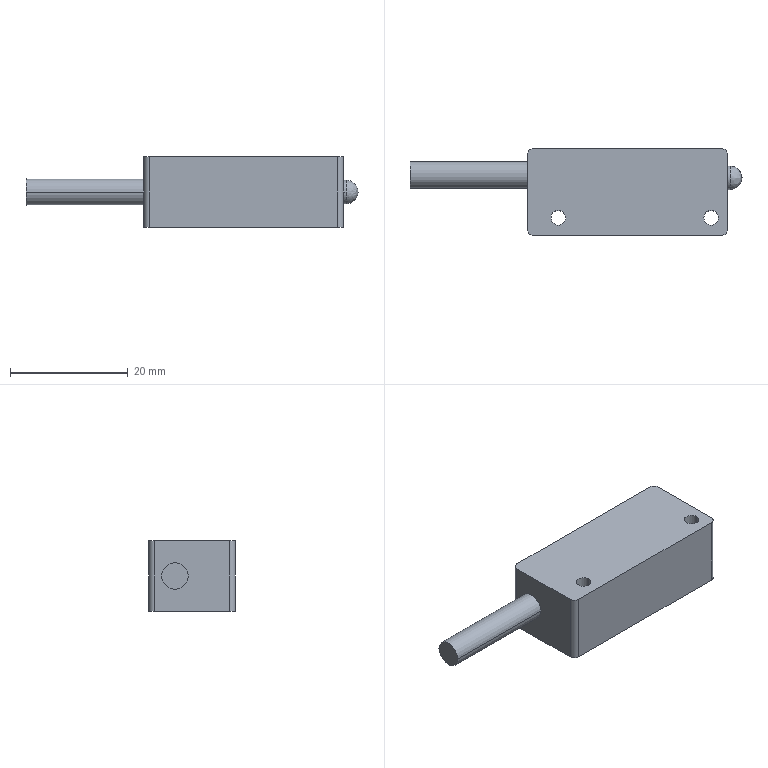Part | SolidWorks | features BaseBody 1 | 1 solid | 20 faces | box 56.42 x 14.8 x 12 mm | volume 6251 mm3 | cylinder 12 | plane 7 | spline 1 | commonest cylinder face diameters 2 x4 2.5 x4 4 x2 4.5 x2
STEP:
#1=CARTESIAN_POINT('',(-13.,-4.4,-6.));
#2=VERTEX_POINT('',#1);
#3=CARTESIAN_POINT('',(-10.5,-4.4,-6.));
#4=VERTEX_POINT('',#3);
#5=CARTESIAN_POINT('',(-11.75,-4.4,-6.));
#6=DIRECTION('',(0.,0.,1.));
#7=DIRECTION('',(1.,0.,0.));
#8=AXIS2_PLACEMENT_3D('',#5,#6,#7);
#9=CIRCLE('',#8,1.25);
#10=EDGE_CURVE('',#2,#4,#9,.T.);
#11=ORIENTED_EDGE('',*,*,#10,.F.);
#12=CARTESIAN_POINT('',(-13.,-4.4,6.));
#13=VERTEX_POINT('',#12);
#14=CARTESIAN_POINT('',(-13.,-4.4,5.));
#15=DIRECTION('',(0.,0.,1.));
#16=VECTOR('',#15,1000.);
#17=LINE('',#14,#16);
#18=EDGE_CURVE('',#2,#13,#17,.T.);
#19=ORIENTED_EDGE('',*,*,#18,.T.);
#20=CARTESIAN_POINT('',(-10.5,-4.4,6.));
#21=VERTEX_POINT('',#20);
#22=CARTESIAN_POINT('',(-11.75,-4.4,6.));
#23=DIRECTION('',(0.,0.,-1.));
#24=DIRECTION('',(1.,0.,0.));
#25=AXIS2_PLACEMENT_3D('',#22,#23,#24);
#26=CIRCLE('',#25,1.25);
#27=EDGE_CURVE('',#21,#13,#26,.T.);
#28=ORIENTED_EDGE('',*,*,#27,.F.);
#29=CARTESIAN_POINT('',(-10.5,-4.4,5.));
#30=DIRECTION('',(0.,0.,1.));
#31=VECTOR('',#30,1000.);
#32=LINE('',#29,#31);
#33=EDGE_CURVE('',#4,#21,#32,.T.);
#34=ORIENTED_EDGE('',*,*,#33,.F.);
#35=EDGE_LOOP('',(#11,#19,#28,#34));
#36=FACE_OUTER_BOUND('',#35,.T.);
#37=CARTESIAN_POINT('',(-11.75,-4.4,5.));
#38=DIRECTION('',(0.,0.,1.));
#39=DIRECTION('',(1.,0.,0.));
#40=AXIS2_PLACEMENT_3D('',#37,#38,#39);
#41=CYLINDRICAL_SURFACE('',#40,1.25);
#42=ADVANCED_FACE('',(#36),#41,.F.);
#43=CARTESIAN_POINT('',(13.,-4.4,-6.));
#44=VERTEX_POINT('',#43);
#45=CARTESIAN_POINT('',(15.5,-4.4,-6.));
#46=VERTEX_POINT('',#45);
#47=CARTESIAN_POINT('',(14.25,-4.4,-6.));
#48=DIRECTION('',(0.,0.,1.));
#49=DIRECTION('',(1.,0.,0.));
#50=AXIS2_PLACEMENT_3D('',#47,#48,#49);
#51=CIRCLE('',#50,1.25);
#52=EDGE_CURVE('',#44,#46,#51,.T.);
#53=ORIENTED_EDGE('',*,*,#52,.F.);
#54=CARTESIAN_POINT('',(13.,-4.4,6.));
#55=VERTEX_POINT('',#54);
#56=CARTESIAN_POINT('',(13.,-4.4,5.));
#57=DIRECTION('',(0.,0.,1.));
#58=VECTOR('',#57,1000.);
#59=LINE('',#56,#58);
#60=EDGE_CURVE('',#44,#55,#59,.T.);
#61=ORIENTED_EDGE('',*,*,#60,.T.);
#62=CARTESIAN_POINT('',(15.5,-4.4,6.));
#63=VERTEX_POINT('',#62);
#64=CARTESIAN_POINT('',(14.25,-4.4,6.));
#65=DIRECTION('',(0.,0.,-1.));
#66=DIRECTION('',(1.,0.,0.));
#67=AXIS2_PLACEMENT_3D('',#64,#65,#66);
#68=CIRCLE('',#67,1.25);
#69=EDGE_CURVE('',#63,#55,#68,.T.);
#70=ORIENTED_EDGE('',*,*,#69,.F.);
#71=CARTESIAN_POINT('',(15.5,-4.4,5.));
#72=DIRECTION('',(0.,0.,1.));
#73=VECTOR('',#72,1000.);
#74=LINE('',#71,#73);
#75=EDGE_CURVE('',#46,#63,#74,.T.);
#76=ORIENTED_EDGE('',*,*,#75,.F.);
#77=EDGE_LOOP('',(#53,#61,#70,#76));
#78=FACE_OUTER_BOUND('',#77,.T.);
#79=CARTESIAN_POINT('',(14.25,-4.4,5.));
#80=DIRECTION('',(0.,0.,1.));
#81=DIRECTION('',(1.,0.,0.));
#82=AXIS2_PLACEMENT_3D('',#79,#80,#81);
#83=CYLINDRICAL_SURFACE('',#82,1.25);
#84=ADVANCED_FACE('',(#78),#83,.F.);
#85=CARTESIAN_POINT('',(-37.,5.15,0.));
#86=VERTEX_POINT('',#85);
#87=CARTESIAN_POINT('',(-37.,0.65,0.));
#88=VERTEX_POINT('',#87);
#89=CARTESIAN_POINT('',(-37.,2.9,0.));
#90=DIRECTION('',(1.,0.,0.));
#91=DIRECTION('',(0.,1.,0.));
#92=AXIS2_PLACEMENT_3D('',#89,#90,#91);
#93=CIRCLE('',#92,2.25);
#94=EDGE_CURVE('',#86,#88,#93,.T.);
#95=ORIENTED_EDGE('',*,*,#94,.T.);
#96=CARTESIAN_POINT('',(-17.,0.65,0.));
#97=VERTEX_POINT('',#96);
#98=CARTESIAN_POINT('',(-37.,0.65,0.));
#99=DIRECTION('',(1.,0.,0.));
#100=VECTOR('',#99,1000.);
#101=LINE('',#98,#100);
#102=EDGE_CURVE('',#88,#97,#101,.T.);
#103=ORIENTED_EDGE('',*,*,#102,.T.);
#104=CARTESIAN_POINT('',(-17.,5.15,0.));
#105=VERTEX_POINT('',#104);
#106=CARTESIAN_POINT('',(-17.,2.9,0.));
#107=DIRECTION('',(-1.,0.,0.));
#108=DIRECTION('',(0.,1.,0.));
#109=AXIS2_PLACEMENT_3D('',#106,#107,#108);
#110=CIRCLE('',#109,2.25);
#111=EDGE_CURVE('',#97,#105,#110,.T.);
#112=ORIENTED_EDGE('',*,*,#111,.T.);
#113=CARTESIAN_POINT('',(-37.,5.15,0.));
#114=DIRECTION('',(1.,0.,0.));
#115=VECTOR('',#114,1000.);
#116=LINE('',#113,#115);
#117=EDGE_CURVE('',#86,#105,#116,.T.);
#118=ORIENTED_EDGE('',*,*,#117,.F.);
#119=EDGE_LOOP('',(#95,#103,#112,#118));
#120=FACE_OUTER_BOUND('',#119,.T.);
#121=CARTESIAN_POINT('',(-37.,2.9,0.));
#122=DIRECTION('',(1.,0.,0.));
#123=DIRECTION('',(0.,1.,0.));
#124=AXIS2_PLACEMENT_3D('',#121,#122,#123);
#125=CYLINDRICAL_SURFACE('',#124,2.25);
#126=ADVANCED_FACE('',(#120),#125,.T.);
#127=CARTESIAN_POINT('',(17.5,2.4,2.));
#128=VERTEX_POINT('',#127);
#129=CARTESIAN_POINT('',(17.5,4.4,0.));
#130=VERTEX_POINT('',#129);
#131=CARTESIAN_POINT('',(17.5,2.4,0.));
#132=DIRECTION('',(-1.,0.,0.));
#133=DIRECTION('',(0.,-1.,0.));
#134=AXIS2_PLACEMENT_3D('',#131,#132,#133);
#135=CIRCLE('',#134,2.);
#136=EDGE_CURVE('',#128,#130,#135,.T.);
#137=ORIENTED_EDGE('',*,*,#136,.T.);
#138=CARTESIAN_POINT('',(17.,4.4,0.));
#139=VERTEX_POINT('',#138);
#140=CARTESIAN_POINT('',(17.5,4.4,0.));
#141=DIRECTION('',(-1.,0.,0.));
#142=VECTOR('',#141,1000.);
#143=LINE('',#140,#142);
#144=EDGE_CURVE('',#130,#139,#143,.T.);
#145=ORIENTED_EDGE('',*,*,#144,.T.);
#146=CARTESIAN_POINT('',(17.,0.4,0.));
#147=VERTEX_POINT('',#146);
#148=CARTESIAN_POINT('',(17.,2.4,0.));
#149=DIRECTION('',(1.,0.,0.));
#150=DIRECTION('',(0.,-1.,0.));
#151=AXIS2_PLACEMENT_3D('',#148,#149,#150);
#152=CIRCLE('',#151,2.);
#153=EDGE_CURVE('',#139,#147,#152,.T.);
#154=ORIENTED_EDGE('',*,*,#153,.T.);
#155=CARTESIAN_POINT('',(17.5,0.4,0.));
#156=VERTEX_POINT('',#155);
#157=CARTESIAN_POINT('',(17.5,0.4,0.));
#158=DIRECTION('',(-1.,0.,0.));
#159=VECTOR('',#158,1000.);
#160=LINE('',#157,#159);
#161=EDGE_CURVE('',#156,#147,#160,.T.);
#162=ORIENTED_EDGE('',*,*,#161,.F.);
#163=CARTESIAN_POINT('',(17.5,2.4,0.));
#164=DIRECTION('',(-1.,0.,0.));
#165=DIRECTION('',(0.,-1.,0.));
#166=AXIS2_PLACEMENT_3D('',#163,#164,#165);
#167=CIRCLE('',#166,2.);
#168=EDGE_CURVE('',#156,#128,#167,.T.);
#169=ORIENTED_EDGE('',*,*,#168,.T.);
#170=EDGE_LOOP('',(#137,#145,#154,#162,#169));
#171=FACE_OUTER_BOUND('',#170,.T.);
#172=CARTESIAN_POINT('',(17.5,2.4,0.));
#173=DIRECTION('',(-1.,0.,0.));
#174=DIRECTION('',(0.,-1.,0.));
#175=AXIS2_PLACEMENT_3D('',#172,#173,#174);
#176=CYLINDRICAL_SURFACE('',#175,2.);
#177=ADVANCED_FACE('',(#171),#176,.T.);
#178=ORIENTED_EDGE('',*,*,#27,.T.);
#179=CARTESIAN_POINT('',(-11.75,-4.4,6.));
#180=DIRECTION('',(0.,0.,-1.));
#181=DIRECTION('',(1.,0.,0.));
#182=AXIS2_PLACEMENT_3D('',#179,#180,#181);
#183=CIRCLE('',#182,1.25);
#184=EDGE_CURVE('',#13,#21,#183,.T.);
#185=ORIENTED_EDGE('',*,*,#184,.T.);
#186=EDGE_LOOP('',(#178,#185));
#187=FACE_BOUND('',#186,.T.);
#188=CARTESIAN_POINT('',(-16.,-7.4,6.));
#189=VERTEX_POINT('',#188);
#190=CARTESIAN_POINT('',(-17.,-6.4,6.));
#191=VERTEX_POINT('',#190);
#192=CARTESIAN_POINT('',(-16.,-6.4,6.));
#193=DIRECTION('',(0.,0.,-1.));
#194=DIRECTION('',(-1.,0.,0.));
#195=AXIS2_PLACEMENT_3D('',#192,#193,#194);
#196=CIRCLE('',#195,1.);
#197=EDGE_CURVE('',#189,#191,#196,.T.);
#198=ORIENTED_EDGE('',*,*,#197,.F.);
#199=CARTESIAN_POINT('',(16.,-7.4,6.));
#200=VERTEX_POINT('',#199);
#201=CARTESIAN_POINT('',(16.,-7.4,6.));
#202=DIRECTION('',(1.,0.,0.));
#203=VECTOR('',#202,1000.);
#204=LINE('',#201,#203);
#205=EDGE_CURVE('',#189,#200,#204,.T.);
#206=ORIENTED_EDGE('',*,*,#205,.T.);
#207=CARTESIAN_POINT('',(17.,-6.4,6.));
#208=VERTEX_POINT('',#207);
#209=CARTESIAN_POINT('',(16.,-6.4,6.));
#210=DIRECTION('',(0.,0.,-1.));
#211=DIRECTION('',(-1.,0.,0.));
#212=AXIS2_PLACEMENT_3D('',#209,#210,#211);
#213=CIRCLE('',#212,1.);
#214=EDGE_CURVE('',#208,#200,#213,.T.);
#215=ORIENTED_EDGE('',*,*,#214,.F.);
#216=CARTESIAN_POINT('',(17.,6.4,6.));
#217=VERTEX_POINT('',#216);
#218=CARTESIAN_POINT('',(17.,-6.4,6.));
#219=DIRECTION('',(0.,1.,0.));
#220=VECTOR('',#219,1000.);
#221=LINE('',#218,#220);
#222=EDGE_CURVE('',#208,#217,#221,.T.);
#223=ORIENTED_EDGE('',*,*,#222,.T.);
#224=CARTESIAN_POINT('',(16.,7.4,6.));
#225=VERTEX_POINT('',#224);
#226=CARTESIAN_POINT('',(16.,6.4,6.));
#227=DIRECTION('',(0.,0.,-1.));
#228=DIRECTION('',(-1.,0.,0.));
#229=AXIS2_PLACEMENT_3D('',#226,#227,#228);
#230=CIRCLE('',#229,1.);
#231=EDGE_CURVE('',#225,#217,#230,.T.);
#232=ORIENTED_EDGE('',*,*,#231,.F.);
#233=CARTESIAN_POINT('',(-16.,7.4,6.));
#234=VERTEX_POINT('',#233);
#235=CARTESIAN_POINT('',(16.,7.4,6.));
#236=DIRECTION('',(-1.,0.,0.));
#237=VECTOR('',#236,1000.);
#238=LINE('',#235,#237);
#239=EDGE_CURVE('',#225,#234,#238,.T.);
#240=ORIENTED_EDGE('',*,*,#239,.T.);
#241=CARTESIAN_POINT('',(-17.,6.4,6.));
#242=VERTEX_POINT('',#241);
#243=CARTESIAN_POINT('',(-16.,6.4,6.));
#244=DIRECTION('',(0.,0.,-1.));
#245=DIRECTION('',(-1.,0.,0.));
#246=AXIS2_PLACEMENT_3D('',#243,#244,#245);
#247=CIRCLE('',#246,1.);
#248=EDGE_CURVE('',#242,#234,#247,.T.);
#249=ORIENTED_EDGE('',*,*,#248,.F.);
#250=CARTESIAN_POINT('',(-17.,-6.4,6.));
#251=DIRECTION('',(0.,-1.,0.));
#252=VECTOR('',#251,1000.);
#253=LINE('',#250,#252);
#254=EDGE_CURVE('',#242,#191,#253,.T.);
#255=ORIENTED_EDGE('',*,*,#254,.T.);
#256=EDGE_LOOP('',(#198,#206,#215,#223,#232,#240,#249,#255));
#257=FACE_OUTER_BOUND('',#256,.T.);
#258=ORIENTED_EDGE('',*,*,#69,.T.);
#259=CARTESIAN_POINT('',(14.25,-4.4,6.));
#260=DIRECTION('',(0.,0.,-1.));
#261=DIRECTION('',(1.,0.,0.));
#262=AXIS2_PLACEMENT_3D('',#259,#260,#261);
#263=CIRCLE('',#262,1.25);
#264=EDGE_CURVE('',#55,#63,#263,.T.);
#265=ORIENTED_EDGE('',*,*,#264,.T.);
#266=EDGE_LOOP('',(#258,#265));
#267=FACE_BOUND('',#266,.T.);
#268=CARTESIAN_POINT('',(16.,-6.4,6.));
#269=DIRECTION('',(0.,0.,1.));
#270=DIRECTION('',(1.,0.,0.));
#271=AXIS2_PLACEMENT_3D('',#268,#269,#270);
#272=PLANE('',#271);
#273=ADVANCED_FACE('',(#187,#257,#267),#272,.T.);
#274=ORIENTED_EDGE('',*,*,#18,.F.);
#275=CARTESIAN_POINT('',(-11.75,-4.4,-6.));
#276=DIRECTION('',(0.,0.,1.));
#277=DIRECTION('',(1.,0.,0.));
#278=AXIS2_PLACEMENT_3D('',#275,#276,#277);
#279=CIRCLE('',#278,1.25);
#280=EDGE_CURVE('',#4,#2,#279,.T.);
#281=ORIENTED_EDGE('',*,*,#280,.F.);
#282=ORIENTED_EDGE('',*,*,#33,.T.);
#283=ORIENTED_EDGE('',*,*,#184,.F.);
#284=EDGE_LOOP('',(#274,#281,#282,#283));
#285=FACE_OUTER_BOUND('',#284,.T.);
#286=CARTESIAN_POINT('',(-11.75,-4.4,5.));
#287=DIRECTION('',(0.,0.,1.));
#288=DIRECTION('',(1.,0.,0.));
#289=AXIS2_PLACEMENT_3D('',#286,#287,#288);
#290=CYLINDRICAL_SURFACE('',#289,1.25);
#291=ADVANCED_FACE('',(#285),#290,.F.);
#292=CARTESIAN_POINT('',(16.,-7.4,-6.));
#293=VERTEX_POINT('',#292);
#294=CARTESIAN_POINT('',(-16.,-7.4,-6.));
#295=VERTEX_POINT('',#294);
#296=CARTESIAN_POINT('',(-17.,-7.4,-6.));
#297=DIRECTION('',(-1.,0.,0.));
#298=VECTOR('',#297,1000.);
#299=LINE('',#296,#298);
#300=EDGE_CURVE('',#293,#295,#299,.T.);
#301=ORIENTED_EDGE('',*,*,#300,.F.);
#302=CARTESIAN_POINT('',(16.,-7.4,5.));
#303=DIRECTION('',(0.,0.,-1.));
#304=VECTOR('',#303,1000.);
#305=LINE('',#302,#304);
#306=EDGE_CURVE('',#200,#293,#305,.T.);
#307=ORIENTED_EDGE('',*,*,#306,.F.);
#308=ORIENTED_EDGE('',*,*,#205,.F.);
#309=CARTESIAN_POINT('',(-16.,-7.4,5.));
#310=DIRECTION('',(0.,0.,1.));
#311=VECTOR('',#310,1000.);
#312=LINE('',#309,#311);
#313=EDGE_CURVE('',#295,#189,#312,.T.);
#314=ORIENTED_EDGE('',*,*,#313,.F.);
#315=EDGE_LOOP('',(#301,#307,#308,#314));
#316=FACE_OUTER_BOUND('',#315,.T.);
#317=CARTESIAN_POINT('',(-17.,-7.4,5.));
#318=DIRECTION('',(0.,1.,0.));
#319=DIRECTION('',(0.,0.,1.));
#320=AXIS2_PLACEMENT_3D('',#317,#318,#319);
#321=PLANE('',#320);
#322=ADVANCED_FACE('',(#316),#321,.F.);
#323=CARTESIAN_POINT('',(-17.,2.9,0.));
#324=DIRECTION('',(-1.,0.,0.));
#325=DIRECTION('',(0.,1.,0.));
#326=AXIS2_PLACEMENT_3D('',#323,#324,#325);
#327=CIRCLE('',#326,2.25);
#328=EDGE_CURVE('',#105,#97,#327,.T.);
#329=ORIENTED_EDGE('',*,*,#328,.F.);
#330=ORIENTED_EDGE('',*,*,#111,.F.);
#331=EDGE_LOOP('',(#329,#330));
#332=FACE_BOUND('',#331,.T.);
#333=ORIENTED_EDGE('',*,*,#254,.F.);
#334=CARTESIAN_POINT('',(-17.,6.4,-6.));
#335=VERTEX_POINT('',#334);
#336=CARTESIAN_POINT('',(-17.,6.4,5.));
#337=DIRECTION('',(0.,0.,1.));
#338=VECTOR('',#337,1000.);
#339=LINE('',#336,#338);
#340=EDGE_CURVE('',#335,#242,#339,.T.);
#341=ORIENTED_EDGE('',*,*,#340,.F.);
#342=CARTESIAN_POINT('',(-17.,-6.4,-6.));
#343=VERTEX_POINT('',#342);
#344=CARTESIAN_POINT('',(-17.,7.4,-6.));
#345=DIRECTION('',(0.,1.,0.));
#346=VECTOR('',#345,1000.);
#347=LINE('',#344,#346);
#348=EDGE_CURVE('',#343,#335,#347,.T.);
#349=ORIENTED_EDGE('',*,*,#348,.F.);
#350=CARTESIAN_POINT('',(-17.,-6.4,5.));
#351=DIRECTION('',(0.,0.,-1.));
#352=VECTOR('',#351,1000.);
#353=LINE('',#350,#352);
#354=EDGE_CURVE('',#191,#343,#353,.T.);
#355=ORIENTED_EDGE('',*,*,#354,.F.);
#356=EDGE_LOOP('',(#333,#341,#349,#355));
#357=FACE_OUTER_BOUND('',#356,.T.);
#358=CARTESIAN_POINT('',(-17.,7.4,5.));
#359=DIRECTION('',(1.,0.,0.));
#360=DIRECTION('',(0.,1.,0.));
#361=AXIS2_PLACEMENT_3D('',#358,#359,#360);
#362=PLANE('',#361);
#363=ADVANCED_FACE('',(#332,#357),#362,.F.);
#364=CARTESIAN_POINT('',(-16.,7.4,-6.));
#365=VERTEX_POINT('',#364);
#366=CARTESIAN_POINT('',(16.,7.4,-6.));
#367=VERTEX_POINT('',#366);
#368=CARTESIAN_POINT('',(-17.,7.4,-6.));
#369=DIRECTION('',(1.,0.,0.));
#370=VECTOR('',#369,1000.);
#371=LINE('',#368,#370);
#372=EDGE_CURVE('',#365,#367,#371,.T.);
#373=ORIENTED_EDGE('',*,*,#372,.F.);
#374=CARTESIAN_POINT('',(-16.,7.4,5.));
#375=DIRECTION('',(0.,0.,-1.));
#376=VECTOR('',#375,1000.);
#377=LINE('',#374,#376);
#378=EDGE_CURVE('',#234,#365,#377,.T.);
#379=ORIENTED_EDGE('',*,*,#378,.F.);
#380=ORIENTED_EDGE('',*,*,#239,.F.);
#381=CARTESIAN_POINT('',(16.,7.4,5.));
#382=DIRECTION('',(0.,0.,1.));
#383=VECTOR('',#382,1000.);
#384=LINE('',#381,#383);
#385=EDGE_CURVE('',#367,#225,#384,.T.);
#386=ORIENTED_EDGE('',*,*,#385,.F.);
#387=EDGE_LOOP('',(#373,#379,#380,#386));
#388=FACE_OUTER_BOUND('',#387,.T.);
#389=CARTESIAN_POINT('',(-17.,7.4,5.));
#390=DIRECTION('',(0.,-1.,0.));
#391=DIRECTION('',(0.,0.,-1.));
#392=AXIS2_PLACEMENT_3D('',#389,#390,#391);
#393=PLANE('',#392);
#394=ADVANCED_FACE('',(#388),#393,.F.);
#395=CARTESIAN_POINT('',(17.,2.4,0.));
#396=DIRECTION('',(1.,0.,0.));
#397=DIRECTION('',(0.,-1.,0.));
#398=AXIS2_PLACEMENT_3D('',#395,#396,#397);
#399=CIRCLE('',#398,2.);
#400=EDGE_CURVE('',#147,#139,#399,.T.);
#401=ORIENTED_EDGE('',*,*,#400,.F.);
#402=ORIENTED_EDGE('',*,*,#153,.F.);
#403=EDGE_LOOP('',(#401,#402));
#404=FACE_BOUND('',#403,.T.);
#405=CARTESIAN_POINT('',(17.,6.4,-6.));
#406=VERTEX_POINT('',#405);
#407=CARTESIAN_POINT('',(17.,-6.4,-6.));
#408=VERTEX_POINT('',#407);
#409=CARTESIAN_POINT('',(17.,7.4,-6.));
#410=DIRECTION('',(0.,-1.,0.));
#411=VECTOR('',#410,1000.);
#412=LINE('',#409,#411);
#413=EDGE_CURVE('',#406,#408,#412,.T.);
#414=ORIENTED_EDGE('',*,*,#413,.F.);
#415=CARTESIAN_POINT('',(17.,6.4,5.));
#416=DIRECTION('',(0.,0.,-1.));
#417=VECTOR('',#416,1000.);
#418=LINE('',#415,#417);
#419=EDGE_CURVE('',#217,#406,#418,.T.);
#420=ORIENTED_EDGE('',*,*,#419,.F.);
#421=ORIENTED_EDGE('',*,*,#222,.F.);
#422=CARTESIAN_POINT('',(17.,-6.4,5.));
#423=DIRECTION('',(0.,0.,1.));
#424=VECTOR('',#423,1000.);
#425=LINE('',#422,#424);
#426=EDGE_CURVE('',#408,#208,#425,.T.);
#427=ORIENTED_EDGE('',*,*,#426,.F.);
#428=EDGE_LOOP('',(#414,#420,#421,#427));
#429=FACE_OUTER_BOUND('',#428,.T.);
#430=CARTESIAN_POINT('',(17.,7.4,5.));
#431=DIRECTION('',(-1.,0.,0.));
#432=DIRECTION('',(0.,-1.,0.));
#433=AXIS2_PLACEMENT_3D('',#430,#431,#432);
#434=PLANE('',#433);
#435=ADVANCED_FACE('',(#404,#429),#434,.F.);
#436=ORIENTED_EDGE('',*,*,#60,.F.);
#437=CARTESIAN_POINT('',(14.25,-4.4,-6.));
#438=DIRECTION('',(0.,0.,1.));
#439=DIRECTION('',(1.,0.,0.));
#440=AXIS2_PLACEMENT_3D('',#437,#438,#439);
#441=CIRCLE('',#440,1.25);
#442=EDGE_CURVE('',#46,#44,#441,.T.);
#443=ORIENTED_EDGE('',*,*,#442,.F.);
#444=ORIENTED_EDGE('',*,*,#75,.T.);
#445=ORIENTED_EDGE('',*,*,#264,.F.);
#446=EDGE_LOOP('',(#436,#443,#444,#445));
#447=FACE_OUTER_BOUND('',#446,.T.);
#448=CARTESIAN_POINT('',(14.25,-4.4,5.));
#449=DIRECTION('',(0.,0.,1.));
#450=DIRECTION('',(1.,0.,0.));
#451=AXIS2_PLACEMENT_3D('',#448,#449,#450);
#452=CYLINDRICAL_SURFACE('',#451,1.25);
#453=ADVANCED_FACE('',(#447),#452,.F.);
#454=ORIENTED_EDGE('',*,*,#442,.T.);
#455=ORIENTED_EDGE('',*,*,#52,.T.);
#456=EDGE_LOOP('',(#454,#455));
#457=FACE_BOUND('',#456,.T.);
#458=CARTESIAN_POINT('',(16.,-6.4,-6.));
#459=DIRECTION('',(0.,0.,-1.));
#460=DIRECTION('',(-1.,0.,0.));
#461=AXIS2_PLACEMENT_3D('',#458,#459,#460);
#462=CIRCLE('',#461,1.);
#463=EDGE_CURVE('',#408,#293,#462,.T.);
#464=ORIENTED_EDGE('',*,*,#463,.T.);
#465=ORIENTED_EDGE('',*,*,#300,.T.);
#466=CARTESIAN_POINT('',(-16.,-6.4,-6.));
#467=DIRECTION('',(0.,0.,-1.));
#468=DIRECTION('',(-1.,0.,0.));
#469=AXIS2_PLACEMENT_3D('',#466,#467,#468);
#470=CIRCLE('',#469,1.);
#471=EDGE_CURVE('',#295,#343,#470,.T.);
#472=ORIENTED_EDGE('',*,*,#471,.T.);
#473=ORIENTED_EDGE('',*,*,#348,.T.);
#474=CARTESIAN_POINT('',(-16.,6.4,-6.));
#475=DIRECTION('',(0.,0.,-1.));
#476=DIRECTION('',(-1.,0.,0.));
#477=AXIS2_PLACEMENT_3D('',#474,#475,#476);
#478=CIRCLE('',#477,1.);
#479=EDGE_CURVE('',#335,#365,#478,.T.);
#480=ORIENTED_EDGE('',*,*,#479,.T.);
#481=ORIENTED_EDGE('',*,*,#372,.T.);
#482=CARTESIAN_POINT('',(16.,6.4,-6.));
#483=DIRECTION('',(0.,0.,-1.));
#484=DIRECTION('',(-1.,0.,0.));
#485=AXIS2_PLACEMENT_3D('',#482,#483,#484);
#486=CIRCLE('',#485,1.);
#487=EDGE_CURVE('',#367,#406,#486,.T.);
#488=ORIENTED_EDGE('',*,*,#487,.T.);
#489=ORIENTED_EDGE('',*,*,#413,.T.);
#490=EDGE_LOOP('',(#464,#465,#472,#473,#480,#481,#488,#489));
#491=FACE_OUTER_BOUND('',#490,.T.);
#492=ORIENTED_EDGE('',*,*,#280,.T.);
#493=ORIENTED_EDGE('',*,*,#10,.T.);
#494=EDGE_LOOP('',(#492,#493));
#495=FACE_BOUND('',#494,.T.);
#496=CARTESIAN_POINT('',(-16.,-6.4,-6.));
#497=DIRECTION('',(0.,0.,-1.));
#498=DIRECTION('',(-1.,0.,0.));
#499=AXIS2_PLACEMENT_3D('',#496,#497,#498);
#500=PLANE('',#499);
#501=ADVANCED_FACE('',(#457,#491,#495),#500,.T.);
#502=ORIENTED_EDGE('',*,*,#354,.T.);
#503=ORIENTED_EDGE('',*,*,#471,.F.);
#504=ORIENTED_EDGE('',*,*,#313,.T.);
#505=ORIENTED_EDGE('',*,*,#197,.T.);
#506=EDGE_LOOP('',(#502,#503,#504,#505));
#507=FACE_OUTER_BOUND('',#506,.T.);
#508=CARTESIAN_POINT('',(-16.,-6.4,5.));
#509=DIRECTION('',(0.,0.,-1.));
#510=DIRECTION('',(-1.,0.,0.));
#511=AXIS2_PLACEMENT_3D('',#508,#509,#510);
#512=CYLINDRICAL_SURFACE('',#511,1.);
#513=ADVANCED_FACE('',(#507),#512,.T.);
#514=ORIENTED_EDGE('',*,*,#306,.T.);
#515=ORIENTED_EDGE('',*,*,#463,.F.);
#516=ORIENTED_EDGE('',*,*,#426,.T.);
#517=ORIENTED_EDGE('',*,*,#214,.T.);
#518=EDGE_LOOP('',(#514,#515,#516,#517));
#519=FACE_OUTER_BOUND('',#518,.T.);
#520=CARTESIAN_POINT('',(16.,-6.4,5.));
#521=DIRECTION('',(0.,0.,-1.));
#522=DIRECTION('',(-1.,0.,0.));
#523=AXIS2_PLACEMENT_3D('',#520,#521,#522);
#524=CYLINDRICAL_SURFACE('',#523,1.);
#525=ADVANCED_FACE('',(#519),#524,.T.);
#526=ORIENTED_EDGE('',*,*,#102,.F.);
#527=CARTESIAN_POINT('',(-37.,2.9,0.));
#528=DIRECTION('',(1.,0.,0.));
#529=DIRECTION('',(0.,1.,0.));
#530=AXIS2_PLACEMENT_3D('',#527,#528,#529);
#531=CIRCLE('',#530,2.25);
#532=EDGE_CURVE('',#88,#86,#531,.T.);
#533=ORIENTED_EDGE('',*,*,#532,.T.);
#534=ORIENTED_EDGE('',*,*,#117,.T.);
#535=ORIENTED_EDGE('',*,*,#328,.T.);
#536=EDGE_LOOP('',(#526,#533,#534,#535));
#537=FACE_OUTER_BOUND('',#536,.T.);
#538=CARTESIAN_POINT('',(-37.,2.9,0.));
#539=DIRECTION('',(1.,0.,0.));
#540=DIRECTION('',(0.,1.,0.));
#541=AXIS2_PLACEMENT_3D('',#538,#539,#540);
#542=CYLINDRICAL_SURFACE('',#541,2.25);
#543=ADVANCED_FACE('',(#537),#542,.T.);
#544=ORIENTED_EDGE('',*,*,#378,.T.);
#545=ORIENTED_EDGE('',*,*,#479,.F.);
#546=ORIENTED_EDGE('',*,*,#340,.T.);
#547=ORIENTED_EDGE('',*,*,#248,.T.);
#548=EDGE_LOOP('',(#544,#545,#546,#547));
#549=FACE_OUTER_BOUND('',#548,.T.);
#550=CARTESIAN_POINT('',(-16.,6.4,5.));
#551=DIRECTION('',(0.,0.,-1.));
#552=DIRECTION('',(-1.,0.,0.));
#553=AXIS2_PLACEMENT_3D('',#550,#551,#552);
#554=CYLINDRICAL_SURFACE('',#553,1.);
#555=ADVANCED_FACE('',(#549),#554,.T.);
#556=ORIENTED_EDGE('',*,*,#419,.T.);
#557=ORIENTED_EDGE('',*,*,#487,.F.);
#558=ORIENTED_EDGE('',*,*,#385,.T.);
#559=ORIENTED_EDGE('',*,*,#231,.T.);
#560=EDGE_LOOP('',(#556,#557,#558,#559));
#561=FACE_OUTER_BOUND('',#560,.T.);
#562=CARTESIAN_POINT('',(16.,6.4,5.));
#563=DIRECTION('',(0.,0.,-1.));
#564=DIRECTION('',(-1.,0.,0.));
#565=AXIS2_PLACEMENT_3D('',#562,#563,#564);
#566=CYLINDRICAL_SURFACE('',#565,1.);
#567=ADVANCED_FACE('',(#561),#566,.T.);
#568=ORIENTED_EDGE('',*,*,#144,.F.);
#569=CARTESIAN_POINT('',(17.5,2.4,-2.));
#570=VERTEX_POINT('',#569);
#571=CARTESIAN_POINT('',(17.5,2.4,0.));
#572=DIRECTION('',(-1.,0.,0.));
#573=DIRECTION('',(0.,-1.,0.));
#574=AXIS2_PLACEMENT_3D('',#571,#572,#573);
#575=CIRCLE('',#574,2.);
#576=EDGE_CURVE('',#130,#570,#575,.T.);
#577=ORIENTED_EDGE('',*,*,#576,.T.);
#578=CARTESIAN_POINT('',(17.5,2.4,0.));
#579=DIRECTION('',(-1.,0.,0.));
#580=DIRECTION('',(0.,-1.,0.));
#581=AXIS2_PLACEMENT_3D('',#578,#579,#580);
#582=CIRCLE('',#581,2.);
#583=EDGE_CURVE('',#570,#156,#582,.T.);
#584=ORIENTED_EDGE('',*,*,#583,.T.);
#585=ORIENTED_EDGE('',*,*,#161,.T.);
#586=ORIENTED_EDGE('',*,*,#400,.T.);
#587=EDGE_LOOP('',(#568,#577,#584,#585,#586));
#588=FACE_OUTER_BOUND('',#587,.T.);
#589=CARTESIAN_POINT('',(17.5,2.4,0.));
#590=DIRECTION('',(-1.,0.,0.));
#591=DIRECTION('',(0.,-1.,0.));
#592=AXIS2_PLACEMENT_3D('',#589,#590,#591);
#593=CYLINDRICAL_SURFACE('',#592,2.);
#594=ADVANCED_FACE('',(#588),#593,.T.);
#595=ORIENTED_EDGE('',*,*,#94,.F.);
#596=ORIENTED_EDGE('',*,*,#532,.F.);
#597=EDGE_LOOP('',(#595,#596));
#598=FACE_OUTER_BOUND('',#597,.T.);
#599=CARTESIAN_POINT('',(-37.,2.9,0.));
#600=DIRECTION('',(-1.,0.,0.));
#601=DIRECTION('',(0.,-1.,0.));
#602=AXIS2_PLACEMENT_3D('',#599,#600,#601);
#603=PLANE('',#602);
#604=ADVANCED_FACE('',(#598),#603,.T.);
#605=ORIENTED_EDGE('',*,*,#136,.F.);
#606=ORIENTED_EDGE('',*,*,#168,.F.);
#607=ORIENTED_EDGE('',*,*,#583,.F.);
#608=ORIENTED_EDGE('',*,*,#576,.F.);
#609=EDGE_LOOP('',(#605,#606,#607,#608));
#610=FACE_OUTER_BOUND('',#609,.T.);
#611=CARTESIAN_POINT('',(17.5,2.4,-2.));
#612=CARTESIAN_POINT('',(17.5,2.4,-2.));
#613=CARTESIAN_POINT('',(17.5,2.4,-2.));
#614=CARTESIAN_POINT('',(17.5,2.4,-2.));
#615=CARTESIAN_POINT('',(17.5,6.4,-2.));
#616=CARTESIAN_POINT('',(25.5,6.4,-2.));
#617=CARTESIAN_POINT('',(25.5,-1.6,-2.));
#618=CARTESIAN_POINT('',(17.5,-1.6,-2.));
#619=CARTESIAN_POINT('',(17.5,6.4,2.));
#620=CARTESIAN_POINT('',(25.5,6.4,2.));
#621=CARTESIAN_POINT('',(25.5,-1.6,2.));
#622=CARTESIAN_POINT('',(17.5,-1.6,2.));
#623=CARTESIAN_POINT('',(17.5,2.4,2.));
#624=CARTESIAN_POINT('',(17.5,2.4,2.));
#625=CARTESIAN_POINT('',(17.5,2.4,2.));
#626=CARTESIAN_POINT('',(17.5,2.4,2.));
#627=(BOUNDED_SURFACE()B_SPLINE_SURFACE(3,3,((#611,#612,#613,#614),(#615,#616,#617,#618),(#619,#620,#621,#622),(#623,#624,#625,#626)),.UNSPECIFIED.,.F.,.F.,.F.)B_SPLINE_SURFACE_WITH_KNOTS((4,4),(4,4),(0.,1.),(0.,1.),.UNSPECIFIED.)GEOMETRIC_REPRESENTATION_ITEM()RATIONAL_B_SPLINE_SURFACE(((1.,0.3333,0.3333,1.),(0.3333,0.1111,0.1111,0.3333),(0.3333,0.1111,0.1111,0.3333),(1.,0.3333,0.3333,1.)))REPRESENTATION_ITEM('')SURFACE());
#628=ADVANCED_FACE('',(#610),#627,.T.);
#629=CLOSED_SHELL('',(#42,#84,#126,#177,#273,#291,#322,#363,#394,#435,#453,#501,#513,#525,#543,#555,#567,#594,#604,#628));
#630=MANIFOLD_SOLID_BREP('',#629);
#631=CARTESIAN_POINT('',(0.,0.,0.));
#632=DIRECTION('',(0.,0.,1.));
#633=DIRECTION('',(1.,0.,0.));
#634=AXIS2_PLACEMENT_3D('',#631,#632,#633);
#635=(LENGTH_UNIT()NAMED_UNIT(*)SI_UNIT(.MILLI.,.METRE.));
#636=UNCERTAINTY_MEASURE_WITH_UNIT(LENGTH_MEASURE(0.00001),#635,'','');
#637=(NAMED_UNIT(*)PLANE_ANGLE_UNIT()SI_UNIT($,.RADIAN.));
#638=(NAMED_UNIT(*)SI_UNIT($,.STERADIAN.)SOLID_ANGLE_UNIT());
#639=(GEOMETRIC_REPRESENTATION_CONTEXT(3)GLOBAL_UNCERTAINTY_ASSIGNED_CONTEXT((#636))GLOBAL_UNIT_ASSIGNED_CONTEXT((#635,#637,#638))REPRESENTATION_CONTEXT('',''));
#640=ADVANCED_BREP_SHAPE_REPRESENTATION('',(#630,#634),#639);